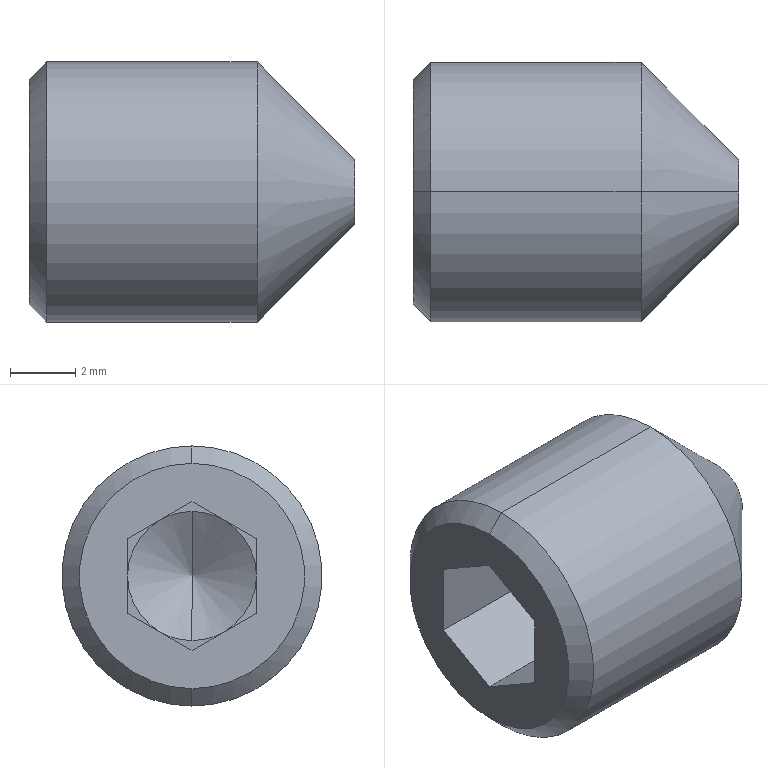Part | SolidWorks | features RevCut 2, Cut 1, LPattern 1, Revolution 1 | 1 solid | 22 faces | box 10 x 8 x 8 mm | volume 368.793 mm3 | plane 14 | cone 6 | cylinder 2 | commonest cylinder face diameters 8 x2
STEP:
#1=CARTESIAN_POINT('',(4.145,0.,0.));
#2=VERTEX_POINT('',#1);
#3=CARTESIAN_POINT('',(3.,0.,1.983));
#4=VERTEX_POINT('',#3);
#5=CARTESIAN_POINT('',(4.145,0.,0.));
#6=DIRECTION('',(-0.5,0.,0.866));
#7=VECTOR('',#6,1000.);
#8=LINE('',#5,#7);
#9=EDGE_CURVE('',#2,#4,#8,.T.);
#10=ORIENTED_EDGE('',*,*,#9,.F.);
#11=CARTESIAN_POINT('',(3.,0.,-1.983));
#12=VERTEX_POINT('',#11);
#13=CARTESIAN_POINT('',(4.145,0.,0.));
#14=DIRECTION('',(-0.5,0.,-0.866));
#15=VECTOR('',#14,1000.);
#16=LINE('',#13,#15);
#17=EDGE_CURVE('',#2,#12,#16,.T.);
#18=ORIENTED_EDGE('',*,*,#17,.T.);
#19=CARTESIAN_POINT('',(3.,-0.9916,-1.718));
#20=VERTEX_POINT('',#19);
#21=CARTESIAN_POINT('',(3.,0.,0.));
#22=DIRECTION('',(-1.,0.,0.));
#23=DIRECTION('',(0.,0.,1.));
#24=AXIS2_PLACEMENT_3D('',#21,#22,#23);
#25=CIRCLE('',#24,1.983);
#26=EDGE_CURVE('',#12,#20,#25,.T.);
#27=ORIENTED_EDGE('',*,*,#26,.T.);
#28=CARTESIAN_POINT('',(3.,-1.983,0.));
#29=VERTEX_POINT('',#28);
#30=CARTESIAN_POINT('',(3.,0.,0.));
#31=DIRECTION('',(-1.,0.,0.));
#32=DIRECTION('',(0.,0.,1.));
#33=AXIS2_PLACEMENT_3D('',#30,#31,#32);
#34=CIRCLE('',#33,1.983);
#35=EDGE_CURVE('',#20,#29,#34,.T.);
#36=ORIENTED_EDGE('',*,*,#35,.T.);
#37=CARTESIAN_POINT('',(3.,-0.9916,1.718));
#38=VERTEX_POINT('',#37);
#39=CARTESIAN_POINT('',(3.,0.,0.));
#40=DIRECTION('',(-1.,0.,0.));
#41=DIRECTION('',(0.,0.,1.));
#42=AXIS2_PLACEMENT_3D('',#39,#40,#41);
#43=CIRCLE('',#42,1.983);
#44=EDGE_CURVE('',#29,#38,#43,.T.);
#45=ORIENTED_EDGE('',*,*,#44,.T.);
#46=CARTESIAN_POINT('',(3.,0.,0.));
#47=DIRECTION('',(-1.,0.,0.));
#48=DIRECTION('',(0.,0.,1.));
#49=AXIS2_PLACEMENT_3D('',#46,#47,#48);
#50=CIRCLE('',#49,1.983);
#51=EDGE_CURVE('',#38,#4,#50,.T.);
#52=ORIENTED_EDGE('',*,*,#51,.T.);
#53=EDGE_LOOP('',(#10,#18,#27,#36,#45,#52));
#54=FACE_OUTER_BOUND('',#53,.T.);
#55=CARTESIAN_POINT('',(-995.855,0.,0.));
#56=DIRECTION('',(-1.,0.,0.));
#57=DIRECTION('',(0.,0.,1.));
#58=AXIS2_PLACEMENT_3D('',#55,#56,#57);
#59=CONICAL_SURFACE('',#58,1732.051,1.047);
#60=ADVANCED_FACE('',(#54),#59,.F.);
#61=CARTESIAN_POINT('',(0.,0.,3.464));
#62=VERTEX_POINT('',#61);
#63=CARTESIAN_POINT('',(0.,0.,-3.464));
#64=VERTEX_POINT('',#63);
#65=CARTESIAN_POINT('',(0.,0.,0.));
#66=DIRECTION('',(-1.,0.,0.));
#67=DIRECTION('',(0.,0.,1.));
#68=AXIS2_PLACEMENT_3D('',#65,#66,#67);
#69=CIRCLE('',#68,3.464);
#70=EDGE_CURVE('',#62,#64,#69,.T.);
#71=ORIENTED_EDGE('',*,*,#70,.F.);
#72=CARTESIAN_POINT('',(0.536,0.,4.));
#73=VERTEX_POINT('',#72);
#74=CARTESIAN_POINT('',(0.536,0.,4.));
#75=DIRECTION('',(0.7071,0.,0.7071));
#76=VECTOR('',#75,1000.);
#77=LINE('',#74,#76);
#78=EDGE_CURVE('',#62,#73,#77,.T.);
#79=ORIENTED_EDGE('',*,*,#78,.T.);
#80=CARTESIAN_POINT('',(0.536,0.,-4.));
#81=VERTEX_POINT('',#80);
#82=CARTESIAN_POINT('',(0.536,0.,0.));
#83=DIRECTION('',(-1.,0.,0.));
#84=DIRECTION('',(0.,0.,1.));
#85=AXIS2_PLACEMENT_3D('',#82,#83,#84);
#86=CIRCLE('',#85,4.);
#87=EDGE_CURVE('',#73,#81,#86,.T.);
#88=ORIENTED_EDGE('',*,*,#87,.T.);
#89=CARTESIAN_POINT('',(0.536,0.,-4.));
#90=DIRECTION('',(0.7071,0.,-0.7071));
#91=VECTOR('',#90,1000.);
#92=LINE('',#89,#91);
#93=EDGE_CURVE('',#64,#81,#92,.T.);
#94=ORIENTED_EDGE('',*,*,#93,.F.);
#95=EDGE_LOOP('',(#71,#79,#88,#94));
#96=FACE_OUTER_BOUND('',#95,.T.);
#97=CARTESIAN_POINT('',(0.536,0.,0.));
#98=DIRECTION('',(1.,0.,0.));
#99=DIRECTION('',(0.,0.,-1.));
#100=AXIS2_PLACEMENT_3D('',#97,#98,#99);
#101=CONICAL_SURFACE('',#100,4.,0.7854);
#102=ADVANCED_FACE('',(#96),#101,.T.);
#103=CARTESIAN_POINT('',(7.,0.,4.));
#104=VERTEX_POINT('',#103);
#105=CARTESIAN_POINT('',(7.,0.,-4.));
#106=VERTEX_POINT('',#105);
#107=CARTESIAN_POINT('',(7.,0.,0.));
#108=DIRECTION('',(-1.,0.,0.));
#109=DIRECTION('',(0.,0.,1.));
#110=AXIS2_PLACEMENT_3D('',#107,#108,#109);
#111=CIRCLE('',#110,4.);
#112=EDGE_CURVE('',#104,#106,#111,.T.);
#113=ORIENTED_EDGE('',*,*,#112,.T.);
#114=CARTESIAN_POINT('',(-1.41,0.,-4.));
#115=DIRECTION('',(-1.,0.,0.));
#116=VECTOR('',#115,1000.);
#117=LINE('',#114,#116);
#118=EDGE_CURVE('',#106,#81,#117,.T.);
#119=ORIENTED_EDGE('',*,*,#118,.T.);
#120=ORIENTED_EDGE('',*,*,#87,.F.);
#121=CARTESIAN_POINT('',(-1.41,0.,4.));
#122=DIRECTION('',(-1.,0.,0.));
#123=VECTOR('',#122,1000.);
#124=LINE('',#121,#123);
#125=EDGE_CURVE('',#104,#73,#124,.T.);
#126=ORIENTED_EDGE('',*,*,#125,.F.);
#127=EDGE_LOOP('',(#113,#119,#120,#126));
#128=FACE_OUTER_BOUND('',#127,.T.);
#129=CARTESIAN_POINT('',(-1.41,0.,0.));
#130=DIRECTION('',(-1.,0.,0.));
#131=DIRECTION('',(0.,0.,1.));
#132=AXIS2_PLACEMENT_3D('',#129,#130,#131);
#133=CYLINDRICAL_SURFACE('',#132,4.);
#134=ADVANCED_FACE('',(#128),#133,.T.);
#135=CARTESIAN_POINT('',(10.,0.,1.));
#136=VERTEX_POINT('',#135);
#137=CARTESIAN_POINT('',(10.,0.,-1.));
#138=VERTEX_POINT('',#137);
#139=CARTESIAN_POINT('',(10.,0.,0.));
#140=DIRECTION('',(-1.,0.,0.));
#141=DIRECTION('',(0.,0.,1.));
#142=AXIS2_PLACEMENT_3D('',#139,#140,#141);
#143=CIRCLE('',#142,1.);
#144=EDGE_CURVE('',#136,#138,#143,.T.);
#145=ORIENTED_EDGE('',*,*,#144,.T.);
#146=CARTESIAN_POINT('',(10.,0.,-1.));
#147=DIRECTION('',(-0.7071,0.,-0.7071));
#148=VECTOR('',#147,1000.);
#149=LINE('',#146,#148);
#150=EDGE_CURVE('',#138,#106,#149,.T.);
#151=ORIENTED_EDGE('',*,*,#150,.T.);
#152=ORIENTED_EDGE('',*,*,#112,.F.);
#153=CARTESIAN_POINT('',(10.,0.,1.));
#154=DIRECTION('',(-0.7071,0.,0.7071));
#155=VECTOR('',#154,1000.);
#156=LINE('',#153,#155);
#157=EDGE_CURVE('',#136,#104,#156,.T.);
#158=ORIENTED_EDGE('',*,*,#157,.F.);
#159=EDGE_LOOP('',(#145,#151,#152,#158));
#160=FACE_OUTER_BOUND('',#159,.T.);
#161=CARTESIAN_POINT('',(10.,0.,0.));
#162=DIRECTION('',(-1.,0.,0.));
#163=DIRECTION('',(0.,0.,1.));
#164=AXIS2_PLACEMENT_3D('',#161,#162,#163);
#165=CONICAL_SURFACE('',#164,1.,0.7854);
#166=ADVANCED_FACE('',(#160),#165,.T.);
#167=CARTESIAN_POINT('',(3.,0.9916,1.718));
#168=VERTEX_POINT('',#167);
#169=CARTESIAN_POINT('',(3.,1.983,0.));
#170=VERTEX_POINT('',#169);
#171=CARTESIAN_POINT('',(3.,0.,0.));
#172=DIRECTION('',(-1.,0.,0.));
#173=DIRECTION('',(0.,0.,1.));
#174=AXIS2_PLACEMENT_3D('',#171,#172,#173);
#175=CIRCLE('',#174,1.983);
#176=EDGE_CURVE('',#168,#170,#175,.T.);
#177=ORIENTED_EDGE('',*,*,#176,.F.);
#178=CARTESIAN_POINT('',(3.,1.983,1.145));
#179=VERTEX_POINT('',#178);
#180=CARTESIAN_POINT('',(3.,0.,2.29));
#181=DIRECTION('',(0.,0.866,-0.5));
#182=VECTOR('',#181,1000.);
#183=LINE('',#180,#182);
#184=EDGE_CURVE('',#168,#179,#183,.T.);
#185=ORIENTED_EDGE('',*,*,#184,.T.);
#186=CARTESIAN_POINT('',(3.,1.983,1.145));
#187=DIRECTION('',(0.,0.,-1.));
#188=VECTOR('',#187,1000.);
#189=LINE('',#186,#188);
#190=EDGE_CURVE('',#179,#170,#189,.T.);
#191=ORIENTED_EDGE('',*,*,#190,.T.);
#192=EDGE_LOOP('',(#177,#185,#191));
#193=FACE_OUTER_BOUND('',#192,.T.);
#194=CARTESIAN_POINT('',(3.,1.983,3.435));
#195=DIRECTION('',(-1.,0.,0.));
#196=DIRECTION('',(0.,0.,1.));
#197=AXIS2_PLACEMENT_3D('',#194,#195,#196);
#198=PLANE('',#197);
#199=ADVANCED_FACE('',(#193),#198,.T.);
#200=CARTESIAN_POINT('',(3.,0.9916,-1.718));
#201=VERTEX_POINT('',#200);
#202=CARTESIAN_POINT('',(3.,0.,0.));
#203=DIRECTION('',(-1.,0.,0.));
#204=DIRECTION('',(0.,0.,1.));
#205=AXIS2_PLACEMENT_3D('',#202,#203,#204);
#206=CIRCLE('',#205,1.983);
#207=EDGE_CURVE('',#170,#201,#206,.T.);
#208=ORIENTED_EDGE('',*,*,#207,.F.);
#209=CARTESIAN_POINT('',(3.,1.983,-1.145));
#210=VERTEX_POINT('',#209);
#211=CARTESIAN_POINT('',(3.,1.983,1.145));
#212=DIRECTION('',(0.,0.,-1.));
#213=VECTOR('',#212,1000.);
#214=LINE('',#211,#213);
#215=EDGE_CURVE('',#170,#210,#214,.T.);
#216=ORIENTED_EDGE('',*,*,#215,.T.);
#217=CARTESIAN_POINT('',(3.,1.983,-1.145));
#218=DIRECTION('',(0.,-0.866,-0.5));
#219=VECTOR('',#218,1000.);
#220=LINE('',#217,#219);
#221=EDGE_CURVE('',#210,#201,#220,.T.);
#222=ORIENTED_EDGE('',*,*,#221,.T.);
#223=EDGE_LOOP('',(#208,#216,#222));
#224=FACE_OUTER_BOUND('',#223,.T.);
#225=CARTESIAN_POINT('',(3.,1.983,3.435));
#226=DIRECTION('',(-1.,0.,0.));
#227=DIRECTION('',(0.,0.,1.));
#228=AXIS2_PLACEMENT_3D('',#225,#226,#227);
#229=PLANE('',#228);
#230=ADVANCED_FACE('',(#224),#229,.T.);
#231=CARTESIAN_POINT('',(3.,0.,0.));
#232=DIRECTION('',(-1.,0.,0.));
#233=DIRECTION('',(0.,0.,1.));
#234=AXIS2_PLACEMENT_3D('',#231,#232,#233);
#235=CIRCLE('',#234,1.983);
#236=EDGE_CURVE('',#201,#12,#235,.T.);
#237=ORIENTED_EDGE('',*,*,#236,.F.);
#238=CARTESIAN_POINT('',(3.,0.,-2.29));
#239=VERTEX_POINT('',#238);
#240=CARTESIAN_POINT('',(3.,1.983,-1.145));
#241=DIRECTION('',(0.,-0.866,-0.5));
#242=VECTOR('',#241,1000.);
#243=LINE('',#240,#242);
#244=EDGE_CURVE('',#201,#239,#243,.T.);
#245=ORIENTED_EDGE('',*,*,#244,.T.);
#246=CARTESIAN_POINT('',(3.,0.,-2.29));
#247=DIRECTION('',(0.,-0.866,0.5));
#248=VECTOR('',#247,1000.);
#249=LINE('',#246,#248);
#250=EDGE_CURVE('',#239,#20,#249,.T.);
#251=ORIENTED_EDGE('',*,*,#250,.T.);
#252=ORIENTED_EDGE('',*,*,#26,.F.);
#253=EDGE_LOOP('',(#237,#245,#251,#252));
#254=FACE_OUTER_BOUND('',#253,.T.);
#255=CARTESIAN_POINT('',(3.,1.983,3.435));
#256=DIRECTION('',(-1.,0.,0.));
#257=DIRECTION('',(0.,0.,1.));
#258=AXIS2_PLACEMENT_3D('',#255,#256,#257);
#259=PLANE('',#258);
#260=ADVANCED_FACE('',(#254),#259,.T.);
#261=ORIENTED_EDGE('',*,*,#35,.F.);
#262=CARTESIAN_POINT('',(3.,-1.983,-1.145));
#263=VERTEX_POINT('',#262);
#264=CARTESIAN_POINT('',(3.,0.,-2.29));
#265=DIRECTION('',(0.,-0.866,0.5));
#266=VECTOR('',#265,1000.);
#267=LINE('',#264,#266);
#268=EDGE_CURVE('',#20,#263,#267,.T.);
#269=ORIENTED_EDGE('',*,*,#268,.T.);
#270=CARTESIAN_POINT('',(3.,-1.983,-1.145));
#271=DIRECTION('',(0.,0.,1.));
#272=VECTOR('',#271,1000.);
#273=LINE('',#270,#272);
#274=EDGE_CURVE('',#263,#29,#273,.T.);
#275=ORIENTED_EDGE('',*,*,#274,.T.);
#276=EDGE_LOOP('',(#261,#269,#275));
#277=FACE_OUTER_BOUND('',#276,.T.);
#278=CARTESIAN_POINT('',(3.,1.983,3.435));
#279=DIRECTION('',(-1.,0.,0.));
#280=DIRECTION('',(0.,0.,1.));
#281=AXIS2_PLACEMENT_3D('',#278,#279,#280);
#282=PLANE('',#281);
#283=ADVANCED_FACE('',(#277),#282,.T.);
#284=ORIENTED_EDGE('',*,*,#44,.F.);
#285=CARTESIAN_POINT('',(3.,-1.983,1.145));
#286=VERTEX_POINT('',#285);
#287=CARTESIAN_POINT('',(3.,-1.983,-1.145));
#288=DIRECTION('',(0.,0.,1.));
#289=VECTOR('',#288,1000.);
#290=LINE('',#287,#289);
#291=EDGE_CURVE('',#29,#286,#290,.T.);
#292=ORIENTED_EDGE('',*,*,#291,.T.);
#293=CARTESIAN_POINT('',(3.,-1.983,1.145));
#294=DIRECTION('',(0.,0.866,0.5));
#295=VECTOR('',#294,1000.);
#296=LINE('',#293,#295);
#297=EDGE_CURVE('',#286,#38,#296,.T.);
#298=ORIENTED_EDGE('',*,*,#297,.T.);
#299=EDGE_LOOP('',(#284,#292,#298));
#300=FACE_OUTER_BOUND('',#299,.T.);
#301=CARTESIAN_POINT('',(3.,1.983,3.435));
#302=DIRECTION('',(-1.,0.,0.));
#303=DIRECTION('',(0.,0.,1.));
#304=AXIS2_PLACEMENT_3D('',#301,#302,#303);
#305=PLANE('',#304);
#306=ADVANCED_FACE('',(#300),#305,.T.);
#307=CARTESIAN_POINT('',(0.,0.,2.29));
#308=VERTEX_POINT('',#307);
#309=CARTESIAN_POINT('',(0.,1.983,1.145));
#310=VERTEX_POINT('',#309);
#311=CARTESIAN_POINT('',(0.,0.,2.29));
#312=DIRECTION('',(0.,0.866,-0.5));
#313=VECTOR('',#312,1000.);
#314=LINE('',#311,#313);
#315=EDGE_CURVE('',#308,#310,#314,.T.);
#316=ORIENTED_EDGE('',*,*,#315,.F.);
#317=CARTESIAN_POINT('',(0.,-1.983,1.145));
#318=VERTEX_POINT('',#317);
#319=CARTESIAN_POINT('',(0.,-1.983,1.145));
#320=DIRECTION('',(0.,0.866,0.5));
#321=VECTOR('',#320,1000.);
#322=LINE('',#319,#321);
#323=EDGE_CURVE('',#318,#308,#322,.T.);
#324=ORIENTED_EDGE('',*,*,#323,.F.);
#325=CARTESIAN_POINT('',(0.,-1.983,-1.145));
#326=VERTEX_POINT('',#325);
#327=CARTESIAN_POINT('',(0.,-1.983,-1.145));
#328=DIRECTION('',(0.,0.,1.));
#329=VECTOR('',#328,1000.);
#330=LINE('',#327,#329);
#331=EDGE_CURVE('',#326,#318,#330,.T.);
#332=ORIENTED_EDGE('',*,*,#331,.F.);
#333=CARTESIAN_POINT('',(0.,0.,-2.29));
#334=VERTEX_POINT('',#333);
#335=CARTESIAN_POINT('',(0.,0.,-2.29));
#336=DIRECTION('',(0.,-0.866,0.5));
#337=VECTOR('',#336,1000.);
#338=LINE('',#335,#337);
#339=EDGE_CURVE('',#334,#326,#338,.T.);
#340=ORIENTED_EDGE('',*,*,#339,.F.);
#341=CARTESIAN_POINT('',(0.,1.983,-1.145));
#342=VERTEX_POINT('',#341);
#343=CARTESIAN_POINT('',(0.,1.983,-1.145));
#344=DIRECTION('',(0.,-0.866,-0.5));
#345=VECTOR('',#344,1000.);
#346=LINE('',#343,#345);
#347=EDGE_CURVE('',#342,#334,#346,.T.);
#348=ORIENTED_EDGE('',*,*,#347,.F.);
#349=CARTESIAN_POINT('',(0.,1.983,1.145));
#350=DIRECTION('',(0.,0.,-1.));
#351=VECTOR('',#350,1000.);
#352=LINE('',#349,#351);
#353=EDGE_CURVE('',#310,#342,#352,.T.);
#354=ORIENTED_EDGE('',*,*,#353,.F.);
#355=EDGE_LOOP('',(#316,#324,#332,#340,#348,#354));
#356=FACE_BOUND('',#355,.T.);
#357=CARTESIAN_POINT('',(0.,0.,0.));
#358=DIRECTION('',(-1.,0.,0.));
#359=DIRECTION('',(0.,0.,1.));
#360=AXIS2_PLACEMENT_3D('',#357,#358,#359);
#361=CIRCLE('',#360,3.464);
#362=EDGE_CURVE('',#64,#62,#361,.T.);
#363=ORIENTED_EDGE('',*,*,#362,.T.);
#364=ORIENTED_EDGE('',*,*,#70,.T.);
#365=EDGE_LOOP('',(#363,#364));
#366=FACE_OUTER_BOUND('',#365,.T.);
#367=CARTESIAN_POINT('',(0.,3.464,0.));
#368=DIRECTION('',(1.,0.,0.));
#369=DIRECTION('',(0.,0.,-1.));
#370=AXIS2_PLACEMENT_3D('',#367,#368,#369);
#371=PLANE('',#370);
#372=ADVANCED_FACE('',(#356,#366),#371,.F.);
#373=ORIENTED_EDGE('',*,*,#144,.F.);
#374=CARTESIAN_POINT('',(10.,0.,0.));
#375=DIRECTION('',(-1.,0.,0.));
#376=DIRECTION('',(0.,0.,1.));
#377=AXIS2_PLACEMENT_3D('',#374,#375,#376);
#378=CIRCLE('',#377,1.);
#379=EDGE_CURVE('',#138,#136,#378,.T.);
#380=ORIENTED_EDGE('',*,*,#379,.F.);
#381=EDGE_LOOP('',(#373,#380));
#382=FACE_OUTER_BOUND('',#381,.T.);
#383=CARTESIAN_POINT('',(10.,0.,0.));
#384=DIRECTION('',(-1.,0.,0.));
#385=DIRECTION('',(0.,0.,1.));
#386=AXIS2_PLACEMENT_3D('',#383,#384,#385);
#387=PLANE('',#386);
#388=ADVANCED_FACE('',(#382),#387,.F.);
#389=ORIENTED_EDGE('',*,*,#150,.F.);
#390=ORIENTED_EDGE('',*,*,#379,.T.);
#391=ORIENTED_EDGE('',*,*,#157,.T.);
#392=CARTESIAN_POINT('',(7.,0.,0.));
#393=DIRECTION('',(-1.,0.,0.));
#394=DIRECTION('',(0.,0.,1.));
#395=AXIS2_PLACEMENT_3D('',#392,#393,#394);
#396=CIRCLE('',#395,4.);
#397=EDGE_CURVE('',#106,#104,#396,.T.);
#398=ORIENTED_EDGE('',*,*,#397,.F.);
#399=EDGE_LOOP('',(#389,#390,#391,#398));
#400=FACE_OUTER_BOUND('',#399,.T.);
#401=CARTESIAN_POINT('',(10.,0.,0.));
#402=DIRECTION('',(-1.,0.,0.));
#403=DIRECTION('',(0.,0.,1.));
#404=AXIS2_PLACEMENT_3D('',#401,#402,#403);
#405=CONICAL_SURFACE('',#404,1.,0.7854);
#406=ADVANCED_FACE('',(#400),#405,.T.);
#407=ORIENTED_EDGE('',*,*,#118,.F.);
#408=ORIENTED_EDGE('',*,*,#397,.T.);
#409=ORIENTED_EDGE('',*,*,#125,.T.);
#410=CARTESIAN_POINT('',(0.536,0.,0.));
#411=DIRECTION('',(-1.,0.,0.));
#412=DIRECTION('',(0.,0.,1.));
#413=AXIS2_PLACEMENT_3D('',#410,#411,#412);
#414=CIRCLE('',#413,4.);
#415=EDGE_CURVE('',#81,#73,#414,.T.);
#416=ORIENTED_EDGE('',*,*,#415,.F.);
#417=EDGE_LOOP('',(#407,#408,#409,#416));
#418=FACE_OUTER_BOUND('',#417,.T.);
#419=CARTESIAN_POINT('',(-1.41,0.,0.));
#420=DIRECTION('',(-1.,0.,0.));
#421=DIRECTION('',(0.,0.,1.));
#422=AXIS2_PLACEMENT_3D('',#419,#420,#421);
#423=CYLINDRICAL_SURFACE('',#422,4.);
#424=ADVANCED_FACE('',(#418),#423,.T.);
#425=ORIENTED_EDGE('',*,*,#78,.F.);
#426=ORIENTED_EDGE('',*,*,#362,.F.);
#427=ORIENTED_EDGE('',*,*,#93,.T.);
#428=ORIENTED_EDGE('',*,*,#415,.T.);
#429=EDGE_LOOP('',(#425,#426,#427,#428));
#430=FACE_OUTER_BOUND('',#429,.T.);
#431=CARTESIAN_POINT('',(0.536,0.,0.));
#432=DIRECTION('',(1.,0.,0.));
#433=DIRECTION('',(0.,0.,-1.));
#434=AXIS2_PLACEMENT_3D('',#431,#432,#433);
#435=CONICAL_SURFACE('',#434,4.,0.7854);
#436=ADVANCED_FACE('',(#430),#435,.T.);
#437=ORIENTED_EDGE('',*,*,#323,.T.);
#438=CARTESIAN_POINT('',(3.,0.,2.29));
#439=VERTEX_POINT('',#438);
#440=CARTESIAN_POINT('',(3.,0.,2.29));
#441=DIRECTION('',(-1.,0.,0.));
#442=VECTOR('',#441,1000.);
#443=LINE('',#440,#442);
#444=EDGE_CURVE('',#439,#308,#443,.T.);
#445=ORIENTED_EDGE('',*,*,#444,.F.);
#446=CARTESIAN_POINT('',(3.,-1.983,1.145));
#447=DIRECTION('',(0.,0.866,0.5));
#448=VECTOR('',#447,1000.);
#449=LINE('',#446,#448);
#450=EDGE_CURVE('',#38,#439,#449,.T.);
#451=ORIENTED_EDGE('',*,*,#450,.F.);
#452=ORIENTED_EDGE('',*,*,#297,.F.);
#453=CARTESIAN_POINT('',(3.,-1.983,1.145));
#454=DIRECTION('',(-1.,0.,0.));
#455=VECTOR('',#454,1000.);
#456=LINE('',#453,#455);
#457=EDGE_CURVE('',#286,#318,#456,.T.);
#458=ORIENTED_EDGE('',*,*,#457,.T.);
#459=EDGE_LOOP('',(#437,#445,#451,#452,#458));
#460=FACE_OUTER_BOUND('',#459,.T.);
#461=CARTESIAN_POINT('',(3.,-1.983,1.145));
#462=DIRECTION('',(0.,-0.5,0.866));
#463=DIRECTION('',(0.,-0.866,-0.5));
#464=AXIS2_PLACEMENT_3D('',#461,#462,#463);
#465=PLANE('',#464);
#466=ADVANCED_FACE('',(#460),#465,.F.);
#467=ORIENTED_EDGE('',*,*,#331,.T.);
#468=ORIENTED_EDGE('',*,*,#457,.F.);
#469=ORIENTED_EDGE('',*,*,#291,.F.);
#470=ORIENTED_EDGE('',*,*,#274,.F.);
#471=CARTESIAN_POINT('',(3.,-1.983,-1.145));
#472=DIRECTION('',(-1.,0.,0.));
#473=VECTOR('',#472,1000.);
#474=LINE('',#471,#473);
#475=EDGE_CURVE('',#263,#326,#474,.T.);
#476=ORIENTED_EDGE('',*,*,#475,.T.);
#477=EDGE_LOOP('',(#467,#468,#469,#470,#476));
#478=FACE_OUTER_BOUND('',#477,.T.);
#479=CARTESIAN_POINT('',(3.,-1.983,-1.145));
#480=DIRECTION('',(0.,-1.,0.));
#481=DIRECTION('',(0.,0.,-1.));
#482=AXIS2_PLACEMENT_3D('',#479,#480,#481);
#483=PLANE('',#482);
#484=ADVANCED_FACE('',(#478),#483,.F.);
#485=ORIENTED_EDGE('',*,*,#339,.T.);
#486=ORIENTED_EDGE('',*,*,#475,.F.);
#487=ORIENTED_EDGE('',*,*,#268,.F.);
#488=ORIENTED_EDGE('',*,*,#250,.F.);
#489=CARTESIAN_POINT('',(3.,0.,-2.29));
#490=DIRECTION('',(-1.,0.,0.));
#491=VECTOR('',#490,1000.);
#492=LINE('',#489,#491);
#493=EDGE_CURVE('',#239,#334,#492,.T.);
#494=ORIENTED_EDGE('',*,*,#493,.T.);
#495=EDGE_LOOP('',(#485,#486,#487,#488,#494));
#496=FACE_OUTER_BOUND('',#495,.T.);
#497=CARTESIAN_POINT('',(3.,0.,-2.29));
#498=DIRECTION('',(0.,-0.5,-0.866));
#499=DIRECTION('',(0.,0.866,-0.5));
#500=AXIS2_PLACEMENT_3D('',#497,#498,#499);
#501=PLANE('',#500);
#502=ADVANCED_FACE('',(#496),#501,.F.);
#503=ORIENTED_EDGE('',*,*,#347,.T.);
#504=ORIENTED_EDGE('',*,*,#493,.F.);
#505=ORIENTED_EDGE('',*,*,#244,.F.);
#506=ORIENTED_EDGE('',*,*,#221,.F.);
#507=CARTESIAN_POINT('',(3.,1.983,-1.145));
#508=DIRECTION('',(-1.,0.,0.));
#509=VECTOR('',#508,1000.);
#510=LINE('',#507,#509);
#511=EDGE_CURVE('',#210,#342,#510,.T.);
#512=ORIENTED_EDGE('',*,*,#511,.T.);
#513=EDGE_LOOP('',(#503,#504,#505,#506,#512));
#514=FACE_OUTER_BOUND('',#513,.T.);
#515=CARTESIAN_POINT('',(3.,1.983,-1.145));
#516=DIRECTION('',(0.,0.5,-0.866));
#517=DIRECTION('',(0.,0.866,0.5));
#518=AXIS2_PLACEMENT_3D('',#515,#516,#517);
#519=PLANE('',#518);
#520=ADVANCED_FACE('',(#514),#519,.F.);
#521=ORIENTED_EDGE('',*,*,#353,.T.);
#522=ORIENTED_EDGE('',*,*,#511,.F.);
#523=ORIENTED_EDGE('',*,*,#215,.F.);
#524=ORIENTED_EDGE('',*,*,#190,.F.);
#525=CARTESIAN_POINT('',(3.,1.983,1.145));
#526=DIRECTION('',(-1.,0.,0.));
#527=VECTOR('',#526,1000.);
#528=LINE('',#525,#527);
#529=EDGE_CURVE('',#179,#310,#528,.T.);
#530=ORIENTED_EDGE('',*,*,#529,.T.);
#531=EDGE_LOOP('',(#521,#522,#523,#524,#530));
#532=FACE_OUTER_BOUND('',#531,.T.);
#533=CARTESIAN_POINT('',(3.,1.983,1.145));
#534=DIRECTION('',(0.,1.,0.));
#535=DIRECTION('',(0.,0.,1.));
#536=AXIS2_PLACEMENT_3D('',#533,#534,#535);
#537=PLANE('',#536);
#538=ADVANCED_FACE('',(#532),#537,.F.);
#539=ORIENTED_EDGE('',*,*,#315,.T.);
#540=ORIENTED_EDGE('',*,*,#529,.F.);
#541=ORIENTED_EDGE('',*,*,#184,.F.);
#542=CARTESIAN_POINT('',(3.,0.,2.29));
#543=DIRECTION('',(0.,0.866,-0.5));
#544=VECTOR('',#543,1000.);
#545=LINE('',#542,#544);
#546=EDGE_CURVE('',#439,#168,#545,.T.);
#547=ORIENTED_EDGE('',*,*,#546,.F.);
#548=ORIENTED_EDGE('',*,*,#444,.T.);
#549=EDGE_LOOP('',(#539,#540,#541,#547,#548));
#550=FACE_OUTER_BOUND('',#549,.T.);
#551=CARTESIAN_POINT('',(3.,0.,2.29));
#552=DIRECTION('',(0.,0.5,0.866));
#553=DIRECTION('',(0.,-0.866,0.5));
#554=AXIS2_PLACEMENT_3D('',#551,#552,#553);
#555=PLANE('',#554);
#556=ADVANCED_FACE('',(#550),#555,.F.);
#557=ORIENTED_EDGE('',*,*,#51,.F.);
#558=ORIENTED_EDGE('',*,*,#450,.T.);
#559=ORIENTED_EDGE('',*,*,#546,.T.);
#560=CARTESIAN_POINT('',(3.,0.,0.));
#561=DIRECTION('',(-1.,0.,0.));
#562=DIRECTION('',(0.,0.,1.));
#563=AXIS2_PLACEMENT_3D('',#560,#561,#562);
#564=CIRCLE('',#563,1.983);
#565=EDGE_CURVE('',#4,#168,#564,.T.);
#566=ORIENTED_EDGE('',*,*,#565,.F.);
#567=EDGE_LOOP('',(#557,#558,#559,#566));
#568=FACE_OUTER_BOUND('',#567,.T.);
#569=CARTESIAN_POINT('',(3.,1.983,3.435));
#570=DIRECTION('',(-1.,0.,0.));
#571=DIRECTION('',(0.,0.,1.));
#572=AXIS2_PLACEMENT_3D('',#569,#570,#571);
#573=PLANE('',#572);
#574=ADVANCED_FACE('',(#568),#573,.T.);
#575=ORIENTED_EDGE('',*,*,#17,.F.);
#576=ORIENTED_EDGE('',*,*,#9,.T.);
#577=ORIENTED_EDGE('',*,*,#565,.T.);
#578=ORIENTED_EDGE('',*,*,#176,.T.);
#579=ORIENTED_EDGE('',*,*,#207,.T.);
#580=ORIENTED_EDGE('',*,*,#236,.T.);
#581=EDGE_LOOP('',(#575,#576,#577,#578,#579,#580));
#582=FACE_OUTER_BOUND('',#581,.T.);
#583=CARTESIAN_POINT('',(-995.855,0.,0.));
#584=DIRECTION('',(-1.,0.,0.));
#585=DIRECTION('',(0.,0.,1.));
#586=AXIS2_PLACEMENT_3D('',#583,#584,#585);
#587=CONICAL_SURFACE('',#586,1732.051,1.047);
#588=ADVANCED_FACE('',(#582),#587,.F.);
#589=CLOSED_SHELL('',(#60,#102,#134,#166,#199,#230,#260,#283,#306,#372,#388,#406,#424,#436,#466,#484,#502,#520,#538,#556,#574,#588));
#590=MANIFOLD_SOLID_BREP('',#589);
#591=CARTESIAN_POINT('',(0.,0.,0.));
#592=DIRECTION('',(0.,0.,1.));
#593=DIRECTION('',(1.,0.,0.));
#594=AXIS2_PLACEMENT_3D('',#591,#592,#593);
#595=(LENGTH_UNIT()NAMED_UNIT(*)SI_UNIT(.MILLI.,.METRE.));
#596=UNCERTAINTY_MEASURE_WITH_UNIT(LENGTH_MEASURE(0.00001),#595,'','');
#597=(NAMED_UNIT(*)PLANE_ANGLE_UNIT()SI_UNIT($,.RADIAN.));
#598=(NAMED_UNIT(*)SI_UNIT($,.STERADIAN.)SOLID_ANGLE_UNIT());
#599=(GEOMETRIC_REPRESENTATION_CONTEXT(3)GLOBAL_UNCERTAINTY_ASSIGNED_CONTEXT((#596))GLOBAL_UNIT_ASSIGNED_CONTEXT((#595,#597,#598))REPRESENTATION_CONTEXT('',''));
#600=ADVANCED_BREP_SHAPE_REPRESENTATION('',(#590,#594),#599);